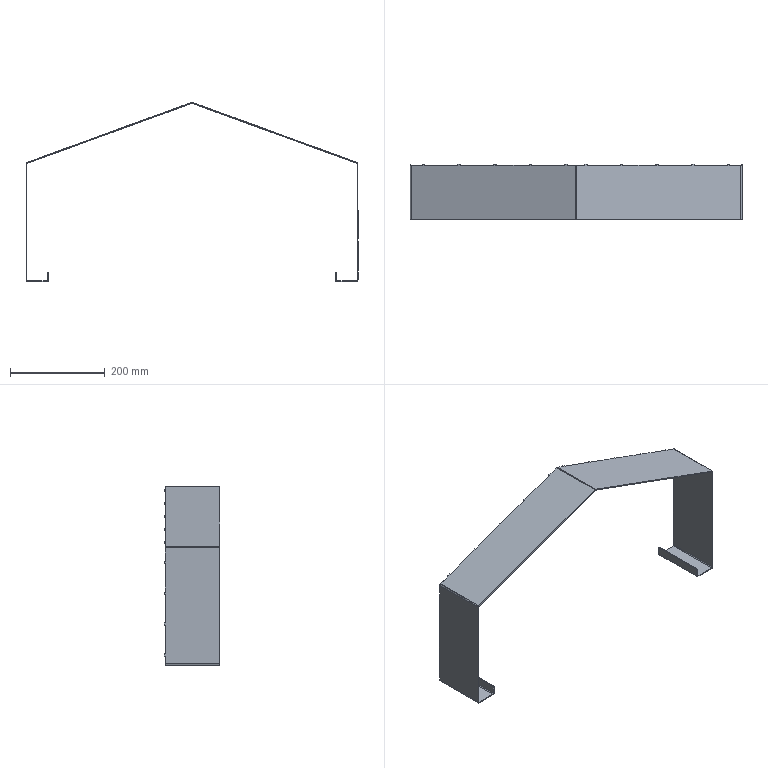Part | NX | features solid 2 | 1 solid | 108 faces | box 700 x 116 x 377.775 mm | volume 311661 mm3 | plane 92 | cylinder 16 | commonest cylinder face diameters 3 x8 7 x8